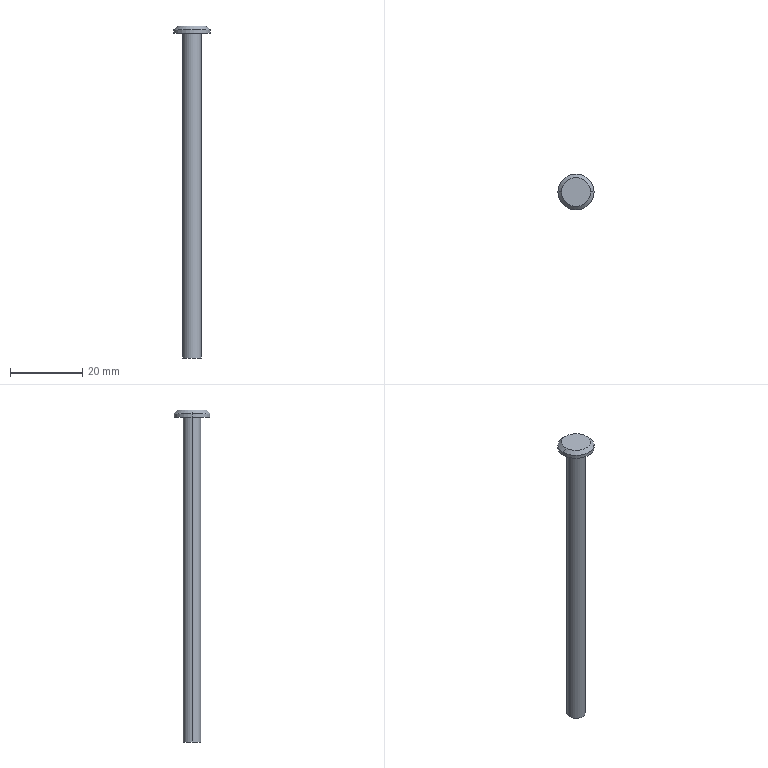Part | SolidWorks | features Chamfer 1, Extrusion 1, ICE 1 | 1 solid | 9 faces | box 10 x 10 x 92 mm | volume 1910 mm3 | cylinder 4 | plane 3 | cone 2 | commonest cylinder face diameters 5 x2 10 x2
STEP:
#1=CARTESIAN_POINT('',(4.,0.,2.));
#2=VERTEX_POINT('',#1);
#3=CARTESIAN_POINT('',(-4.,0.,2.));
#4=VERTEX_POINT('',#3);
#5=CARTESIAN_POINT('',(0.,0.,2.));
#6=DIRECTION('',(0.,0.,1.));
#7=DIRECTION('',(1.,0.,0.));
#8=AXIS2_PLACEMENT_3D('',#5,#6,#7);
#9=CIRCLE('',#8,4.);
#10=EDGE_CURVE('',#2,#4,#9,.T.);
#11=ORIENTED_EDGE('',*,*,#10,.F.);
#12=CARTESIAN_POINT('',(5.,0.,1.));
#13=VERTEX_POINT('',#12);
#14=CARTESIAN_POINT('',(4.,0.,2.));
#15=DIRECTION('',(0.7071,0.,-0.7071));
#16=VECTOR('',#15,1000.);
#17=LINE('',#14,#16);
#18=EDGE_CURVE('',#2,#13,#17,.T.);
#19=ORIENTED_EDGE('',*,*,#18,.T.);
#20=CARTESIAN_POINT('',(-5.,0.,1.));
#21=VERTEX_POINT('',#20);
#22=CARTESIAN_POINT('',(0.,0.,1.));
#23=DIRECTION('',(0.,0.,-1.));
#24=DIRECTION('',(1.,0.,0.));
#25=AXIS2_PLACEMENT_3D('',#22,#23,#24);
#26=CIRCLE('',#25,5.);
#27=EDGE_CURVE('',#21,#13,#26,.T.);
#28=ORIENTED_EDGE('',*,*,#27,.F.);
#29=CARTESIAN_POINT('',(-4.,0.,2.));
#30=DIRECTION('',(-0.7071,0.,-0.7071));
#31=VECTOR('',#30,1000.);
#32=LINE('',#29,#31);
#33=EDGE_CURVE('',#4,#21,#32,.T.);
#34=ORIENTED_EDGE('',*,*,#33,.F.);
#35=EDGE_LOOP('',(#11,#19,#28,#34));
#36=FACE_OUTER_BOUND('',#35,.T.);
#37=CARTESIAN_POINT('',(0.,0.,2.));
#38=DIRECTION('',(0.,0.,-1.));
#39=DIRECTION('',(-1.,0.,0.));
#40=AXIS2_PLACEMENT_3D('',#37,#38,#39);
#41=CONICAL_SURFACE('',#40,4.,0.7854);
#42=ADVANCED_FACE('',(#36),#41,.T.);
#43=CARTESIAN_POINT('',(5.,0.,0.));
#44=VERTEX_POINT('',#43);
#45=CARTESIAN_POINT('',(-5.,0.,0.));
#46=VERTEX_POINT('',#45);
#47=CARTESIAN_POINT('',(0.,0.,0.));
#48=DIRECTION('',(0.,0.,1.));
#49=DIRECTION('',(1.,0.,0.));
#50=AXIS2_PLACEMENT_3D('',#47,#48,#49);
#51=CIRCLE('',#50,5.);
#52=EDGE_CURVE('',#44,#46,#51,.T.);
#53=ORIENTED_EDGE('',*,*,#52,.T.);
#54=CARTESIAN_POINT('',(-5.,0.,0.));
#55=DIRECTION('',(0.,0.,1.));
#56=VECTOR('',#55,1000.);
#57=LINE('',#54,#56);
#58=EDGE_CURVE('',#46,#21,#57,.T.);
#59=ORIENTED_EDGE('',*,*,#58,.T.);
#60=ORIENTED_EDGE('',*,*,#27,.T.);
#61=CARTESIAN_POINT('',(5.,0.,0.));
#62=DIRECTION('',(0.,0.,1.));
#63=VECTOR('',#62,1000.);
#64=LINE('',#61,#63);
#65=EDGE_CURVE('',#44,#13,#64,.T.);
#66=ORIENTED_EDGE('',*,*,#65,.F.);
#67=EDGE_LOOP('',(#53,#59,#60,#66));
#68=FACE_OUTER_BOUND('',#67,.T.);
#69=CARTESIAN_POINT('',(0.,0.,0.));
#70=DIRECTION('',(0.,0.,1.));
#71=DIRECTION('',(1.,0.,0.));
#72=AXIS2_PLACEMENT_3D('',#69,#70,#71);
#73=CYLINDRICAL_SURFACE('',#72,5.);
#74=ADVANCED_FACE('',(#68),#73,.T.);
#75=CARTESIAN_POINT('',(2.5,0.,-90.));
#76=VERTEX_POINT('',#75);
#77=CARTESIAN_POINT('',(-2.5,0.,-90.));
#78=VERTEX_POINT('',#77);
#79=CARTESIAN_POINT('',(0.,0.,-90.));
#80=DIRECTION('',(0.,0.,1.));
#81=DIRECTION('',(1.,0.,0.));
#82=AXIS2_PLACEMENT_3D('',#79,#80,#81);
#83=CIRCLE('',#82,2.5);
#84=EDGE_CURVE('',#76,#78,#83,.T.);
#85=ORIENTED_EDGE('',*,*,#84,.T.);
#86=CARTESIAN_POINT('',(-2.5,0.,0.));
#87=VERTEX_POINT('',#86);
#88=CARTESIAN_POINT('',(-2.5,0.,-90.));
#89=DIRECTION('',(0.,0.,1.));
#90=VECTOR('',#89,1000.);
#91=LINE('',#88,#90);
#92=EDGE_CURVE('',#78,#87,#91,.T.);
#93=ORIENTED_EDGE('',*,*,#92,.T.);
#94=CARTESIAN_POINT('',(2.5,0.,0.));
#95=VERTEX_POINT('',#94);
#96=CARTESIAN_POINT('',(0.,0.,0.));
#97=DIRECTION('',(0.,0.,-1.));
#98=DIRECTION('',(1.,0.,0.));
#99=AXIS2_PLACEMENT_3D('',#96,#97,#98);
#100=CIRCLE('',#99,2.5);
#101=EDGE_CURVE('',#87,#95,#100,.T.);
#102=ORIENTED_EDGE('',*,*,#101,.T.);
#103=CARTESIAN_POINT('',(2.5,0.,-90.));
#104=DIRECTION('',(0.,0.,1.));
#105=VECTOR('',#104,1000.);
#106=LINE('',#103,#105);
#107=EDGE_CURVE('',#76,#95,#106,.T.);
#108=ORIENTED_EDGE('',*,*,#107,.F.);
#109=EDGE_LOOP('',(#85,#93,#102,#108));
#110=FACE_OUTER_BOUND('',#109,.T.);
#111=CARTESIAN_POINT('',(0.,0.,-90.));
#112=DIRECTION('',(0.,0.,1.));
#113=DIRECTION('',(1.,0.,0.));
#114=AXIS2_PLACEMENT_3D('',#111,#112,#113);
#115=CYLINDRICAL_SURFACE('',#114,2.5);
#116=ADVANCED_FACE('',(#110),#115,.T.);
#117=ORIENTED_EDGE('',*,*,#92,.F.);
#118=CARTESIAN_POINT('',(0.,0.,-90.));
#119=DIRECTION('',(0.,0.,1.));
#120=DIRECTION('',(1.,0.,0.));
#121=AXIS2_PLACEMENT_3D('',#118,#119,#120);
#122=CIRCLE('',#121,2.5);
#123=EDGE_CURVE('',#78,#76,#122,.T.);
#124=ORIENTED_EDGE('',*,*,#123,.T.);
#125=ORIENTED_EDGE('',*,*,#107,.T.);
#126=CARTESIAN_POINT('',(0.,0.,0.));
#127=DIRECTION('',(0.,0.,-1.));
#128=DIRECTION('',(1.,0.,0.));
#129=AXIS2_PLACEMENT_3D('',#126,#127,#128);
#130=CIRCLE('',#129,2.5);
#131=EDGE_CURVE('',#95,#87,#130,.T.);
#132=ORIENTED_EDGE('',*,*,#131,.T.);
#133=EDGE_LOOP('',(#117,#124,#125,#132));
#134=FACE_OUTER_BOUND('',#133,.T.);
#135=CARTESIAN_POINT('',(0.,0.,-90.));
#136=DIRECTION('',(0.,0.,1.));
#137=DIRECTION('',(1.,0.,0.));
#138=AXIS2_PLACEMENT_3D('',#135,#136,#137);
#139=CYLINDRICAL_SURFACE('',#138,2.5);
#140=ADVANCED_FACE('',(#134),#139,.T.);
#141=ORIENTED_EDGE('',*,*,#84,.F.);
#142=ORIENTED_EDGE('',*,*,#123,.F.);
#143=EDGE_LOOP('',(#141,#142));
#144=FACE_OUTER_BOUND('',#143,.T.);
#145=CARTESIAN_POINT('',(0.,0.,-90.));
#146=DIRECTION('',(0.,0.,1.));
#147=DIRECTION('',(1.,0.,0.));
#148=AXIS2_PLACEMENT_3D('',#145,#146,#147);
#149=PLANE('',#148);
#150=ADVANCED_FACE('',(#144),#149,.F.);
#151=ORIENTED_EDGE('',*,*,#58,.F.);
#152=CARTESIAN_POINT('',(0.,0.,0.));
#153=DIRECTION('',(0.,0.,1.));
#154=DIRECTION('',(1.,0.,0.));
#155=AXIS2_PLACEMENT_3D('',#152,#153,#154);
#156=CIRCLE('',#155,5.);
#157=EDGE_CURVE('',#46,#44,#156,.T.);
#158=ORIENTED_EDGE('',*,*,#157,.T.);
#159=ORIENTED_EDGE('',*,*,#65,.T.);
#160=CARTESIAN_POINT('',(0.,0.,1.));
#161=DIRECTION('',(0.,0.,-1.));
#162=DIRECTION('',(1.,0.,0.));
#163=AXIS2_PLACEMENT_3D('',#160,#161,#162);
#164=CIRCLE('',#163,5.);
#165=EDGE_CURVE('',#13,#21,#164,.T.);
#166=ORIENTED_EDGE('',*,*,#165,.T.);
#167=EDGE_LOOP('',(#151,#158,#159,#166));
#168=FACE_OUTER_BOUND('',#167,.T.);
#169=CARTESIAN_POINT('',(0.,0.,0.));
#170=DIRECTION('',(0.,0.,1.));
#171=DIRECTION('',(1.,0.,0.));
#172=AXIS2_PLACEMENT_3D('',#169,#170,#171);
#173=CYLINDRICAL_SURFACE('',#172,5.);
#174=ADVANCED_FACE('',(#168),#173,.T.);
#175=ORIENTED_EDGE('',*,*,#131,.F.);
#176=ORIENTED_EDGE('',*,*,#101,.F.);
#177=EDGE_LOOP('',(#175,#176));
#178=FACE_BOUND('',#177,.T.);
#179=ORIENTED_EDGE('',*,*,#52,.F.);
#180=ORIENTED_EDGE('',*,*,#157,.F.);
#181=EDGE_LOOP('',(#179,#180));
#182=FACE_OUTER_BOUND('',#181,.T.);
#183=CARTESIAN_POINT('',(0.,0.,0.));
#184=DIRECTION('',(0.,0.,1.));
#185=DIRECTION('',(1.,0.,0.));
#186=AXIS2_PLACEMENT_3D('',#183,#184,#185);
#187=PLANE('',#186);
#188=ADVANCED_FACE('',(#178,#182),#187,.F.);
#189=CARTESIAN_POINT('',(0.,0.,2.));
#190=DIRECTION('',(0.,0.,1.));
#191=DIRECTION('',(1.,0.,0.));
#192=AXIS2_PLACEMENT_3D('',#189,#190,#191);
#193=CIRCLE('',#192,4.);
#194=EDGE_CURVE('',#4,#2,#193,.T.);
#195=ORIENTED_EDGE('',*,*,#194,.T.);
#196=ORIENTED_EDGE('',*,*,#10,.T.);
#197=EDGE_LOOP('',(#195,#196));
#198=FACE_OUTER_BOUND('',#197,.T.);
#199=CARTESIAN_POINT('',(0.,0.,2.));
#200=DIRECTION('',(0.,0.,1.));
#201=DIRECTION('',(1.,0.,0.));
#202=AXIS2_PLACEMENT_3D('',#199,#200,#201);
#203=PLANE('',#202);
#204=ADVANCED_FACE('',(#198),#203,.T.);
#205=ORIENTED_EDGE('',*,*,#18,.F.);
#206=ORIENTED_EDGE('',*,*,#194,.F.);
#207=ORIENTED_EDGE('',*,*,#33,.T.);
#208=ORIENTED_EDGE('',*,*,#165,.F.);
#209=EDGE_LOOP('',(#205,#206,#207,#208));
#210=FACE_OUTER_BOUND('',#209,.T.);
#211=CARTESIAN_POINT('',(0.,0.,2.));
#212=DIRECTION('',(0.,0.,-1.));
#213=DIRECTION('',(-1.,0.,0.));
#214=AXIS2_PLACEMENT_3D('',#211,#212,#213);
#215=CONICAL_SURFACE('',#214,4.,0.7854);
#216=ADVANCED_FACE('',(#210),#215,.T.);
#217=CLOSED_SHELL('',(#42,#74,#116,#140,#150,#174,#188,#204,#216));
#218=MANIFOLD_SOLID_BREP('',#217);
#219=CARTESIAN_POINT('',(0.,0.,0.));
#220=DIRECTION('',(0.,0.,1.));
#221=DIRECTION('',(1.,0.,0.));
#222=AXIS2_PLACEMENT_3D('',#219,#220,#221);
#223=(LENGTH_UNIT()NAMED_UNIT(*)SI_UNIT(.MILLI.,.METRE.));
#224=UNCERTAINTY_MEASURE_WITH_UNIT(LENGTH_MEASURE(0.00001),#223,'','');
#225=(NAMED_UNIT(*)PLANE_ANGLE_UNIT()SI_UNIT($,.RADIAN.));
#226=(NAMED_UNIT(*)SI_UNIT($,.STERADIAN.)SOLID_ANGLE_UNIT());
#227=(GEOMETRIC_REPRESENTATION_CONTEXT(3)GLOBAL_UNCERTAINTY_ASSIGNED_CONTEXT((#224))GLOBAL_UNIT_ASSIGNED_CONTEXT((#223,#225,#226))REPRESENTATION_CONTEXT('',''));
#228=ADVANCED_BREP_SHAPE_REPRESENTATION('',(#218,#222),#227);